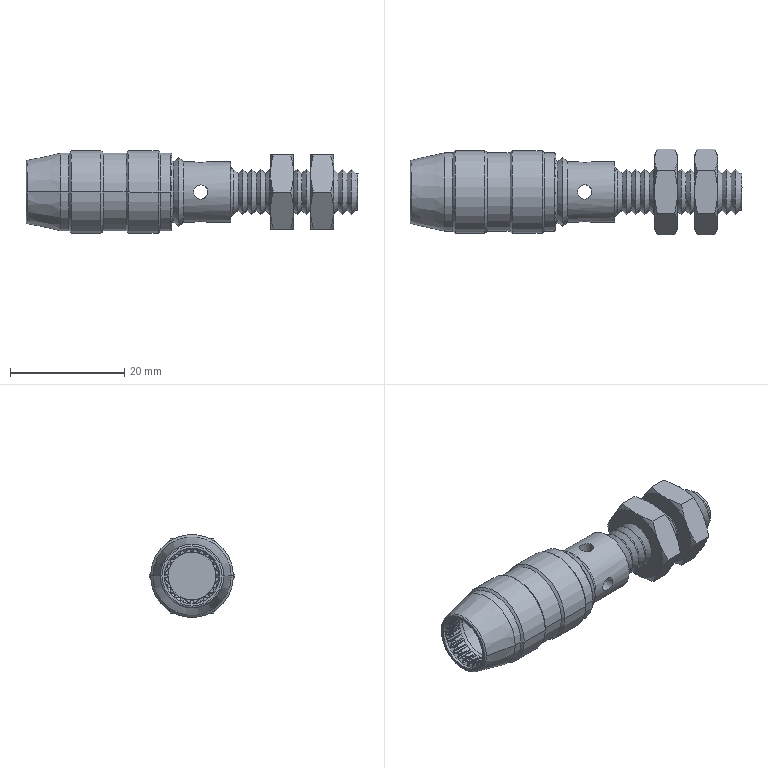Part | STEP file | lll_id4354_x_t | 1 solid | 424 faces | box 58.034 x 15.011 x 14.5 mm | volume 4297 mm3 | cylinder 252 | cone 97 | plane 72 | torus 3 | commonest cylinder face diameters 0.3 x192 8.7 x26 11.15 x6 13.7 x6 2.5 x4 14.5 x4